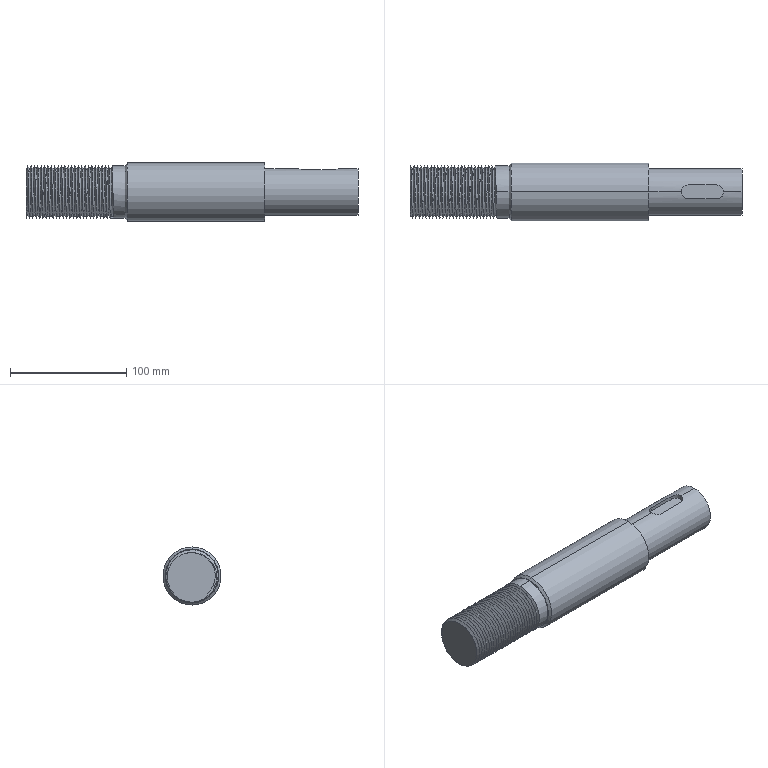Part | SolidWorks | 1 solid | 23 faces | box 285.002 x 50 x 50 mm | volume 456683 mm3 | cylinder 10 | plane 9 | spline 2 | cone 2 | commonest cylinder face diameters 12 x3 45 x3 40 x2 50 x2